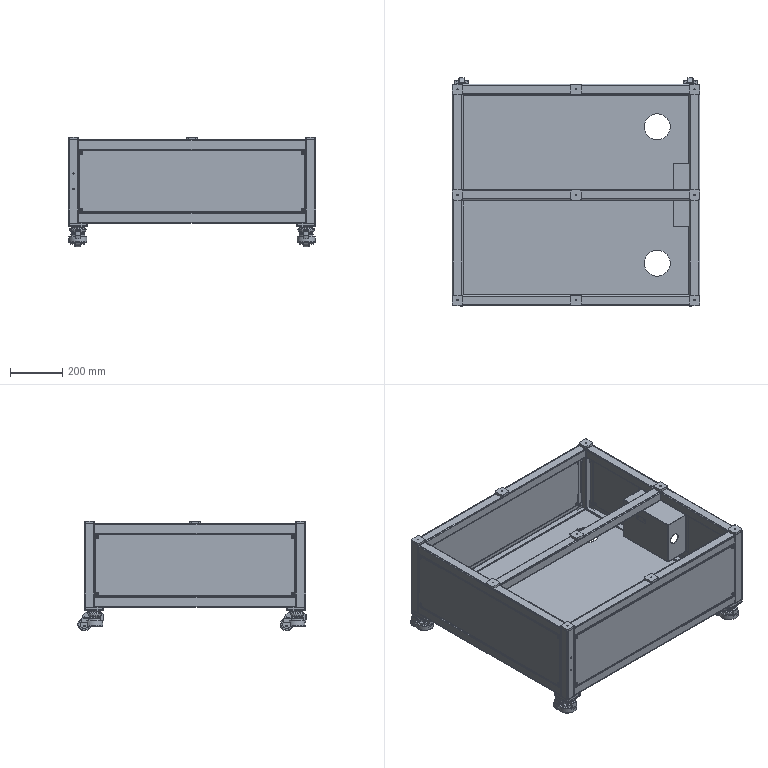Part | SolidWorks | features InContextFeatHolder 11, CompositeCurve 1 | 69 solids | 2672 faces | box 950 x 876 x 421.5 mm | volume 6731533 mm3 | plane 1285 | cylinder 869 | cone 320 | spline 116 | torus 82 | commonest cylinder face diameters 4 x107 10 x102 5 x96 8 x68 5.8 x48 1 x42